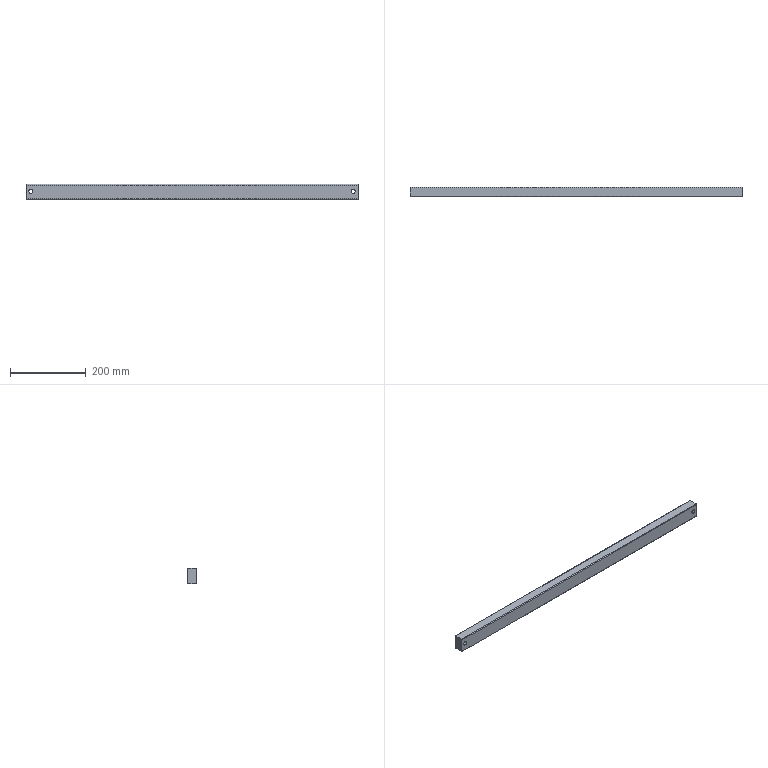Part | SolidWorks | features Cut 1, Fillet 1, Sweep 1, WeldmentFeature 1 | 1 solid | 14 faces | box 875 x 25 x 40 mm | volume 868078 mm3 | cylinder 8 | plane 6 | commonest cylinder face diameters 3.4 x4 11 x4
STEP:
#1=CARTESIAN_POINT('',(830.306,12.5,7.5));
#2=VERTEX_POINT('',#1);
#3=CARTESIAN_POINT('',(830.306,12.5,-3.5));
#4=VERTEX_POINT('',#3);
#5=CARTESIAN_POINT('',(830.306,12.5,2.));
#6=DIRECTION('',(0.,-1.,0.));
#7=DIRECTION('',(0.,0.,1.));
#8=AXIS2_PLACEMENT_3D('',#5,#6,#7);
#9=CIRCLE('',#8,5.5);
#10=EDGE_CURVE('',#2,#4,#9,.T.);
#11=ORIENTED_EDGE('',*,*,#10,.F.);
#12=CARTESIAN_POINT('',(830.306,-12.5,7.5));
#13=VERTEX_POINT('',#12);
#14=CARTESIAN_POINT('',(830.306,12.5,7.5));
#15=DIRECTION('',(0.,-1.,0.));
#16=VECTOR('',#15,1000.);
#17=LINE('',#14,#16);
#18=EDGE_CURVE('',#2,#13,#17,.T.);
#19=ORIENTED_EDGE('',*,*,#18,.T.);
#20=CARTESIAN_POINT('',(830.306,-12.5,-3.5));
#21=VERTEX_POINT('',#20);
#22=CARTESIAN_POINT('',(830.306,-12.5,2.));
#23=DIRECTION('',(0.,-1.,0.));
#24=DIRECTION('',(0.,0.,1.));
#25=AXIS2_PLACEMENT_3D('',#22,#23,#24);
#26=CIRCLE('',#25,5.5);
#27=EDGE_CURVE('',#13,#21,#26,.T.);
#28=ORIENTED_EDGE('',*,*,#27,.T.);
#29=CARTESIAN_POINT('',(830.306,12.5,-3.5));
#30=DIRECTION('',(0.,-1.,0.));
#31=VECTOR('',#30,1000.);
#32=LINE('',#29,#31);
#33=EDGE_CURVE('',#4,#21,#32,.T.);
#34=ORIENTED_EDGE('',*,*,#33,.F.);
#35=EDGE_LOOP('',(#11,#19,#28,#34));
#36=FACE_OUTER_BOUND('',#35,.T.);
#37=CARTESIAN_POINT('',(830.306,12.5,2.));
#38=DIRECTION('',(0.,-1.,0.));
#39=DIRECTION('',(0.,0.,-1.));
#40=AXIS2_PLACEMENT_3D('',#37,#38,#39);
#41=CYLINDRICAL_SURFACE('',#40,5.5);
#42=ADVANCED_FACE('',(#36),#41,.F.);
#43=CARTESIAN_POINT('',(-19.694,12.5,7.5));
#44=VERTEX_POINT('',#43);
#45=CARTESIAN_POINT('',(-19.694,12.5,-3.5));
#46=VERTEX_POINT('',#45);
#47=CARTESIAN_POINT('',(-19.694,12.5,2.));
#48=DIRECTION('',(0.,-1.,0.));
#49=DIRECTION('',(0.,0.,-1.));
#50=AXIS2_PLACEMENT_3D('',#47,#48,#49);
#51=CIRCLE('',#50,5.5);
#52=EDGE_CURVE('',#44,#46,#51,.T.);
#53=ORIENTED_EDGE('',*,*,#52,.F.);
#54=CARTESIAN_POINT('',(-19.694,-12.5,7.5));
#55=VERTEX_POINT('',#54);
#56=CARTESIAN_POINT('',(-19.694,12.5,7.5));
#57=DIRECTION('',(0.,-1.,0.));
#58=VECTOR('',#57,1000.);
#59=LINE('',#56,#58);
#60=EDGE_CURVE('',#44,#55,#59,.T.);
#61=ORIENTED_EDGE('',*,*,#60,.T.);
#62=CARTESIAN_POINT('',(-19.694,-12.5,-3.5));
#63=VERTEX_POINT('',#62);
#64=CARTESIAN_POINT('',(-19.694,-12.5,2.));
#65=DIRECTION('',(0.,-1.,0.));
#66=DIRECTION('',(0.,0.,-1.));
#67=AXIS2_PLACEMENT_3D('',#64,#65,#66);
#68=CIRCLE('',#67,5.5);
#69=EDGE_CURVE('',#55,#63,#68,.T.);
#70=ORIENTED_EDGE('',*,*,#69,.T.);
#71=CARTESIAN_POINT('',(-19.694,12.5,-3.5));
#72=DIRECTION('',(0.,-1.,0.));
#73=VECTOR('',#72,1000.);
#74=LINE('',#71,#73);
#75=EDGE_CURVE('',#46,#63,#74,.T.);
#76=ORIENTED_EDGE('',*,*,#75,.F.);
#77=EDGE_LOOP('',(#53,#61,#70,#76));
#78=FACE_OUTER_BOUND('',#77,.T.);
#79=CARTESIAN_POINT('',(-19.694,12.5,2.));
#80=DIRECTION('',(0.,-1.,0.));
#81=DIRECTION('',(0.,0.,-1.));
#82=AXIS2_PLACEMENT_3D('',#79,#80,#81);
#83=CYLINDRICAL_SURFACE('',#82,5.5);
#84=ADVANCED_FACE('',(#78),#83,.F.);
#85=CARTESIAN_POINT('',(-32.194,10.8,20.));
#86=VERTEX_POINT('',#85);
#87=CARTESIAN_POINT('',(-32.194,-10.8,20.));
#88=VERTEX_POINT('',#87);
#89=CARTESIAN_POINT('',(-32.194,12.5,20.));
#90=DIRECTION('',(0.,-1.,0.));
#91=VECTOR('',#90,1000.);
#92=LINE('',#89,#91);
#93=EDGE_CURVE('',#86,#88,#92,.T.);
#94=ORIENTED_EDGE('',*,*,#93,.T.);
#95=CARTESIAN_POINT('',(842.806,-10.8,20.));
#96=VERTEX_POINT('',#95);
#97=CARTESIAN_POINT('',(842.806,-10.8,20.));
#98=DIRECTION('',(1.,0.,0.));
#99=VECTOR('',#98,1000.);
#100=LINE('',#97,#99);
#101=EDGE_CURVE('',#88,#96,#100,.T.);
#102=ORIENTED_EDGE('',*,*,#101,.T.);
#103=CARTESIAN_POINT('',(842.806,10.8,20.));
#104=VERTEX_POINT('',#103);
#105=CARTESIAN_POINT('',(842.806,12.5,20.));
#106=DIRECTION('',(0.,-1.,0.));
#107=VECTOR('',#106,1000.);
#108=LINE('',#105,#107);
#109=EDGE_CURVE('',#104,#96,#108,.T.);
#110=ORIENTED_EDGE('',*,*,#109,.F.);
#111=CARTESIAN_POINT('',(842.806,10.8,20.));
#112=DIRECTION('',(-1.,0.,0.));
#113=VECTOR('',#112,1000.);
#114=LINE('',#111,#113);
#115=EDGE_CURVE('',#104,#86,#114,.T.);
#116=ORIENTED_EDGE('',*,*,#115,.T.);
#117=EDGE_LOOP('',(#94,#102,#110,#116));
#118=FACE_OUTER_BOUND('',#117,.T.);
#119=CARTESIAN_POINT('',(842.806,12.5,20.));
#120=DIRECTION('',(0.,0.,-1.));
#121=DIRECTION('',(0.,1.,0.));
#122=AXIS2_PLACEMENT_3D('',#119,#120,#121);
#123=PLANE('',#122);
#124=ADVANCED_FACE('',(#118),#123,.F.);
#125=CARTESIAN_POINT('',(830.306,-12.5,2.));
#126=DIRECTION('',(0.,-1.,0.));
#127=DIRECTION('',(0.,0.,1.));
#128=AXIS2_PLACEMENT_3D('',#125,#126,#127);
#129=CIRCLE('',#128,5.5);
#130=EDGE_CURVE('',#21,#13,#129,.T.);
#131=ORIENTED_EDGE('',*,*,#130,.F.);
#132=ORIENTED_EDGE('',*,*,#27,.F.);
#133=EDGE_LOOP('',(#131,#132));
#134=FACE_BOUND('',#133,.T.);
#135=CARTESIAN_POINT('',(-19.694,-12.5,2.));
#136=DIRECTION('',(0.,-1.,0.));
#137=DIRECTION('',(0.,0.,-1.));
#138=AXIS2_PLACEMENT_3D('',#135,#136,#137);
#139=CIRCLE('',#138,5.5);
#140=EDGE_CURVE('',#63,#55,#139,.T.);
#141=ORIENTED_EDGE('',*,*,#140,.F.);
#142=ORIENTED_EDGE('',*,*,#69,.F.);
#143=EDGE_LOOP('',(#141,#142));
#144=FACE_BOUND('',#143,.T.);
#145=CARTESIAN_POINT('',(-32.194,-12.5,18.3));
#146=VERTEX_POINT('',#145);
#147=CARTESIAN_POINT('',(-32.194,-12.5,-18.3));
#148=VERTEX_POINT('',#147);
#149=CARTESIAN_POINT('',(-32.194,-12.5,-20.));
#150=DIRECTION('',(0.,0.,-1.));
#151=VECTOR('',#150,1000.);
#152=LINE('',#149,#151);
#153=EDGE_CURVE('',#146,#148,#152,.T.);
#154=ORIENTED_EDGE('',*,*,#153,.T.);
#155=CARTESIAN_POINT('',(842.806,-12.5,-18.3));
#156=VERTEX_POINT('',#155);
#157=CARTESIAN_POINT('',(842.806,-12.5,-18.3));
#158=DIRECTION('',(1.,0.,0.));
#159=VECTOR('',#158,1000.);
#160=LINE('',#157,#159);
#161=EDGE_CURVE('',#148,#156,#160,.T.);
#162=ORIENTED_EDGE('',*,*,#161,.T.);
#163=CARTESIAN_POINT('',(842.806,-12.5,18.3));
#164=VERTEX_POINT('',#163);
#165=CARTESIAN_POINT('',(842.806,-12.5,-20.));
#166=DIRECTION('',(0.,0.,-1.));
#167=VECTOR('',#166,1000.);
#168=LINE('',#165,#167);
#169=EDGE_CURVE('',#164,#156,#168,.T.);
#170=ORIENTED_EDGE('',*,*,#169,.F.);
#171=CARTESIAN_POINT('',(842.806,-12.5,18.3));
#172=DIRECTION('',(-1.,0.,0.));
#173=VECTOR('',#172,1000.);
#174=LINE('',#171,#173);
#175=EDGE_CURVE('',#164,#146,#174,.T.);
#176=ORIENTED_EDGE('',*,*,#175,.T.);
#177=EDGE_LOOP('',(#154,#162,#170,#176));
#178=FACE_OUTER_BOUND('',#177,.T.);
#179=CARTESIAN_POINT('',(842.806,-12.5,-20.));
#180=DIRECTION('',(0.,1.,0.));
#181=DIRECTION('',(0.,0.,1.));
#182=AXIS2_PLACEMENT_3D('',#179,#180,#181);
#183=PLANE('',#182);
#184=ADVANCED_FACE('',(#134,#144,#178),#183,.F.);
#185=CARTESIAN_POINT('',(842.806,-10.8,-20.));
#186=VERTEX_POINT('',#185);
#187=CARTESIAN_POINT('',(842.806,10.8,-20.));
#188=VERTEX_POINT('',#187);
#189=CARTESIAN_POINT('',(842.806,12.5,-20.));
#190=DIRECTION('',(0.,1.,0.));
#191=VECTOR('',#190,1000.);
#192=LINE('',#189,#191);
#193=EDGE_CURVE('',#186,#188,#192,.T.);
#194=ORIENTED_EDGE('',*,*,#193,.F.);
#195=CARTESIAN_POINT('',(-32.194,-10.8,-20.));
#196=VERTEX_POINT('',#195);
#197=CARTESIAN_POINT('',(842.806,-10.8,-20.));
#198=DIRECTION('',(-1.,0.,0.));
#199=VECTOR('',#198,1000.);
#200=LINE('',#197,#199);
#201=EDGE_CURVE('',#186,#196,#200,.T.);
#202=ORIENTED_EDGE('',*,*,#201,.T.);
#203=CARTESIAN_POINT('',(-32.194,10.8,-20.));
#204=VERTEX_POINT('',#203);
#205=CARTESIAN_POINT('',(-32.194,12.5,-20.));
#206=DIRECTION('',(0.,1.,0.));
#207=VECTOR('',#206,1000.);
#208=LINE('',#205,#207);
#209=EDGE_CURVE('',#196,#204,#208,.T.);
#210=ORIENTED_EDGE('',*,*,#209,.T.);
#211=CARTESIAN_POINT('',(842.806,10.8,-20.));
#212=DIRECTION('',(1.,0.,0.));
#213=VECTOR('',#212,1000.);
#214=LINE('',#211,#213);
#215=EDGE_CURVE('',#204,#188,#214,.T.);
#216=ORIENTED_EDGE('',*,*,#215,.T.);
#217=EDGE_LOOP('',(#194,#202,#210,#216));
#218=FACE_OUTER_BOUND('',#217,.T.);
#219=CARTESIAN_POINT('',(842.806,12.5,-20.));
#220=DIRECTION('',(0.,0.,1.));
#221=DIRECTION('',(0.,-1.,0.));
#222=AXIS2_PLACEMENT_3D('',#219,#220,#221);
#223=PLANE('',#222);
#224=ADVANCED_FACE('',(#218),#223,.F.);
#225=CARTESIAN_POINT('',(830.306,12.5,2.));
#226=DIRECTION('',(0.,-1.,0.));
#227=DIRECTION('',(0.,0.,1.));
#228=AXIS2_PLACEMENT_3D('',#225,#226,#227);
#229=CIRCLE('',#228,5.5);
#230=EDGE_CURVE('',#4,#2,#229,.T.);
#231=ORIENTED_EDGE('',*,*,#230,.T.);
#232=ORIENTED_EDGE('',*,*,#10,.T.);
#233=EDGE_LOOP('',(#231,#232));
#234=FACE_BOUND('',#233,.T.);
#235=CARTESIAN_POINT('',(-19.694,12.5,2.));
#236=DIRECTION('',(0.,-1.,0.));
#237=DIRECTION('',(0.,0.,-1.));
#238=AXIS2_PLACEMENT_3D('',#235,#236,#237);
#239=CIRCLE('',#238,5.5);
#240=EDGE_CURVE('',#46,#44,#239,.T.);
#241=ORIENTED_EDGE('',*,*,#240,.T.);
#242=ORIENTED_EDGE('',*,*,#52,.T.);
#243=EDGE_LOOP('',(#241,#242));
#244=FACE_BOUND('',#243,.T.);
#245=CARTESIAN_POINT('',(-32.194,12.5,-18.3));
#246=VERTEX_POINT('',#245);
#247=CARTESIAN_POINT('',(-32.194,12.5,18.3));
#248=VERTEX_POINT('',#247);
#249=CARTESIAN_POINT('',(-32.194,12.5,-20.));
#250=DIRECTION('',(0.,0.,1.));
#251=VECTOR('',#250,1000.);
#252=LINE('',#249,#251);
#253=EDGE_CURVE('',#246,#248,#252,.T.);
#254=ORIENTED_EDGE('',*,*,#253,.T.);
#255=CARTESIAN_POINT('',(842.806,12.5,18.3));
#256=VERTEX_POINT('',#255);
#257=CARTESIAN_POINT('',(842.806,12.5,18.3));
#258=DIRECTION('',(1.,0.,0.));
#259=VECTOR('',#258,1000.);
#260=LINE('',#257,#259);
#261=EDGE_CURVE('',#248,#256,#260,.T.);
#262=ORIENTED_EDGE('',*,*,#261,.T.);
#263=CARTESIAN_POINT('',(842.806,12.5,-18.3));
#264=VERTEX_POINT('',#263);
#265=CARTESIAN_POINT('',(842.806,12.5,-20.));
#266=DIRECTION('',(0.,0.,1.));
#267=VECTOR('',#266,1000.);
#268=LINE('',#265,#267);
#269=EDGE_CURVE('',#264,#256,#268,.T.);
#270=ORIENTED_EDGE('',*,*,#269,.F.);
#271=CARTESIAN_POINT('',(842.806,12.5,-18.3));
#272=DIRECTION('',(-1.,0.,0.));
#273=VECTOR('',#272,1000.);
#274=LINE('',#271,#273);
#275=EDGE_CURVE('',#264,#246,#274,.T.);
#276=ORIENTED_EDGE('',*,*,#275,.T.);
#277=EDGE_LOOP('',(#254,#262,#270,#276));
#278=FACE_OUTER_BOUND('',#277,.T.);
#279=CARTESIAN_POINT('',(842.806,12.5,-20.));
#280=DIRECTION('',(0.,-1.,0.));
#281=DIRECTION('',(0.,0.,-1.));
#282=AXIS2_PLACEMENT_3D('',#279,#280,#281);
#283=PLANE('',#282);
#284=ADVANCED_FACE('',(#234,#244,#278),#283,.F.);
#285=ORIENTED_EDGE('',*,*,#169,.T.);
#286=CARTESIAN_POINT('',(842.806,-10.8,-18.3));
#287=DIRECTION('',(1.,0.,0.));
#288=DIRECTION('',(0.,0.,1.));
#289=AXIS2_PLACEMENT_3D('',#286,#287,#288);
#290=CIRCLE('',#289,1.7);
#291=EDGE_CURVE('',#156,#186,#290,.T.);
#292=ORIENTED_EDGE('',*,*,#291,.T.);
#293=ORIENTED_EDGE('',*,*,#193,.T.);
#294=CARTESIAN_POINT('',(842.806,10.8,-18.3));
#295=DIRECTION('',(1.,0.,0.));
#296=DIRECTION('',(0.,0.,1.));
#297=AXIS2_PLACEMENT_3D('',#294,#295,#296);
#298=CIRCLE('',#297,1.7);
#299=EDGE_CURVE('',#188,#264,#298,.T.);
#300=ORIENTED_EDGE('',*,*,#299,.T.);
#301=ORIENTED_EDGE('',*,*,#269,.T.);
#302=CARTESIAN_POINT('',(842.806,10.8,18.3));
#303=DIRECTION('',(1.,0.,0.));
#304=DIRECTION('',(0.,0.,1.));
#305=AXIS2_PLACEMENT_3D('',#302,#303,#304);
#306=CIRCLE('',#305,1.7);
#307=EDGE_CURVE('',#256,#104,#306,.T.);
#308=ORIENTED_EDGE('',*,*,#307,.T.);
#309=ORIENTED_EDGE('',*,*,#109,.T.);
#310=CARTESIAN_POINT('',(842.806,-10.8,18.3));
#311=DIRECTION('',(1.,0.,0.));
#312=DIRECTION('',(0.,0.,1.));
#313=AXIS2_PLACEMENT_3D('',#310,#311,#312);
#314=CIRCLE('',#313,1.7);
#315=EDGE_CURVE('',#96,#164,#314,.T.);
#316=ORIENTED_EDGE('',*,*,#315,.T.);
#317=EDGE_LOOP('',(#285,#292,#293,#300,#301,#308,#309,#316));
#318=FACE_OUTER_BOUND('',#317,.T.);
#319=CARTESIAN_POINT('',(842.806,0.,0.));
#320=DIRECTION('',(-1.,0.,0.));
#321=DIRECTION('',(0.,0.,1.));
#322=AXIS2_PLACEMENT_3D('',#319,#320,#321);
#323=PLANE('',#322);
#324=ADVANCED_FACE('',(#318),#323,.F.);
#325=ORIENTED_EDGE('',*,*,#209,.F.);
#326=CARTESIAN_POINT('',(-32.194,-10.8,-18.3));
#327=DIRECTION('',(-1.,0.,0.));
#328=DIRECTION('',(0.,0.,1.));
#329=AXIS2_PLACEMENT_3D('',#326,#327,#328);
#330=CIRCLE('',#329,1.7);
#331=EDGE_CURVE('',#196,#148,#330,.T.);
#332=ORIENTED_EDGE('',*,*,#331,.T.);
#333=ORIENTED_EDGE('',*,*,#153,.F.);
#334=CARTESIAN_POINT('',(-32.194,-10.8,18.3));
#335=DIRECTION('',(-1.,0.,0.));
#336=DIRECTION('',(0.,0.,1.));
#337=AXIS2_PLACEMENT_3D('',#334,#335,#336);
#338=CIRCLE('',#337,1.7);
#339=EDGE_CURVE('',#146,#88,#338,.T.);
#340=ORIENTED_EDGE('',*,*,#339,.T.);
#341=ORIENTED_EDGE('',*,*,#93,.F.);
#342=CARTESIAN_POINT('',(-32.194,10.8,18.3));
#343=DIRECTION('',(-1.,0.,0.));
#344=DIRECTION('',(0.,0.,1.));
#345=AXIS2_PLACEMENT_3D('',#342,#343,#344);
#346=CIRCLE('',#345,1.7);
#347=EDGE_CURVE('',#86,#248,#346,.T.);
#348=ORIENTED_EDGE('',*,*,#347,.T.);
#349=ORIENTED_EDGE('',*,*,#253,.F.);
#350=CARTESIAN_POINT('',(-32.194,10.8,-18.3));
#351=DIRECTION('',(-1.,0.,0.));
#352=DIRECTION('',(0.,0.,1.));
#353=AXIS2_PLACEMENT_3D('',#350,#351,#352);
#354=CIRCLE('',#353,1.7);
#355=EDGE_CURVE('',#246,#204,#354,.T.);
#356=ORIENTED_EDGE('',*,*,#355,.T.);
#357=EDGE_LOOP('',(#325,#332,#333,#340,#341,#348,#349,#356));
#358=FACE_OUTER_BOUND('',#357,.T.);
#359=CARTESIAN_POINT('',(-32.194,0.,0.));
#360=DIRECTION('',(-1.,0.,0.));
#361=DIRECTION('',(0.,0.,1.));
#362=AXIS2_PLACEMENT_3D('',#359,#360,#361);
#363=PLANE('',#362);
#364=ADVANCED_FACE('',(#358),#363,.T.);
#365=ORIENTED_EDGE('',*,*,#291,.F.);
#366=ORIENTED_EDGE('',*,*,#161,.F.);
#367=ORIENTED_EDGE('',*,*,#331,.F.);
#368=ORIENTED_EDGE('',*,*,#201,.F.);
#369=EDGE_LOOP('',(#365,#366,#367,#368));
#370=FACE_OUTER_BOUND('',#369,.T.);
#371=CARTESIAN_POINT('',(842.806,-10.8,-18.3));
#372=DIRECTION('',(-1.,0.,0.));
#373=DIRECTION('',(0.,0.,1.));
#374=AXIS2_PLACEMENT_3D('',#371,#372,#373);
#375=CYLINDRICAL_SURFACE('',#374,1.7);
#376=ADVANCED_FACE('',(#370),#375,.T.);
#377=ORIENTED_EDGE('',*,*,#315,.F.);
#378=ORIENTED_EDGE('',*,*,#101,.F.);
#379=ORIENTED_EDGE('',*,*,#339,.F.);
#380=ORIENTED_EDGE('',*,*,#175,.F.);
#381=EDGE_LOOP('',(#377,#378,#379,#380));
#382=FACE_OUTER_BOUND('',#381,.T.);
#383=CARTESIAN_POINT('',(842.806,-10.8,18.3));
#384=DIRECTION('',(-1.,0.,0.));
#385=DIRECTION('',(0.,0.,1.));
#386=AXIS2_PLACEMENT_3D('',#383,#384,#385);
#387=CYLINDRICAL_SURFACE('',#386,1.7);
#388=ADVANCED_FACE('',(#382),#387,.T.);
#389=ORIENTED_EDGE('',*,*,#307,.F.);
#390=ORIENTED_EDGE('',*,*,#261,.F.);
#391=ORIENTED_EDGE('',*,*,#347,.F.);
#392=ORIENTED_EDGE('',*,*,#115,.F.);
#393=EDGE_LOOP('',(#389,#390,#391,#392));
#394=FACE_OUTER_BOUND('',#393,.T.);
#395=CARTESIAN_POINT('',(842.806,10.8,18.3));
#396=DIRECTION('',(-1.,0.,0.));
#397=DIRECTION('',(0.,0.,1.));
#398=AXIS2_PLACEMENT_3D('',#395,#396,#397);
#399=CYLINDRICAL_SURFACE('',#398,1.7);
#400=ADVANCED_FACE('',(#394),#399,.T.);
#401=ORIENTED_EDGE('',*,*,#299,.F.);
#402=ORIENTED_EDGE('',*,*,#215,.F.);
#403=ORIENTED_EDGE('',*,*,#355,.F.);
#404=ORIENTED_EDGE('',*,*,#275,.F.);
#405=EDGE_LOOP('',(#401,#402,#403,#404));
#406=FACE_OUTER_BOUND('',#405,.T.);
#407=CARTESIAN_POINT('',(842.806,10.8,-18.3));
#408=DIRECTION('',(-1.,0.,0.));
#409=DIRECTION('',(0.,0.,1.));
#410=AXIS2_PLACEMENT_3D('',#407,#408,#409);
#411=CYLINDRICAL_SURFACE('',#410,1.7);
#412=ADVANCED_FACE('',(#406),#411,.T.);
#413=ORIENTED_EDGE('',*,*,#60,.F.);
#414=ORIENTED_EDGE('',*,*,#240,.F.);
#415=ORIENTED_EDGE('',*,*,#75,.T.);
#416=ORIENTED_EDGE('',*,*,#140,.T.);
#417=EDGE_LOOP('',(#413,#414,#415,#416));
#418=FACE_OUTER_BOUND('',#417,.T.);
#419=CARTESIAN_POINT('',(-19.694,12.5,2.));
#420=DIRECTION('',(0.,-1.,0.));
#421=DIRECTION('',(0.,0.,-1.));
#422=AXIS2_PLACEMENT_3D('',#419,#420,#421);
#423=CYLINDRICAL_SURFACE('',#422,5.5);
#424=ADVANCED_FACE('',(#418),#423,.F.);
#425=ORIENTED_EDGE('',*,*,#18,.F.);
#426=ORIENTED_EDGE('',*,*,#230,.F.);
#427=ORIENTED_EDGE('',*,*,#33,.T.);
#428=ORIENTED_EDGE('',*,*,#130,.T.);
#429=EDGE_LOOP('',(#425,#426,#427,#428));
#430=FACE_OUTER_BOUND('',#429,.T.);
#431=CARTESIAN_POINT('',(830.306,12.5,2.));
#432=DIRECTION('',(0.,-1.,0.));
#433=DIRECTION('',(0.,0.,-1.));
#434=AXIS2_PLACEMENT_3D('',#431,#432,#433);
#435=CYLINDRICAL_SURFACE('',#434,5.5);
#436=ADVANCED_FACE('',(#430),#435,.F.);
#437=CLOSED_SHELL('',(#42,#84,#124,#184,#224,#284,#324,#364,#376,#388,#400,#412,#424,#436));
#438=MANIFOLD_SOLID_BREP('',#437);
#439=CARTESIAN_POINT('',(0.,0.,0.));
#440=DIRECTION('',(0.,0.,1.));
#441=DIRECTION('',(1.,0.,0.));
#442=AXIS2_PLACEMENT_3D('',#439,#440,#441);
#443=(LENGTH_UNIT()NAMED_UNIT(*)SI_UNIT(.MILLI.,.METRE.));
#444=UNCERTAINTY_MEASURE_WITH_UNIT(LENGTH_MEASURE(0.00001),#443,'','');
#445=(NAMED_UNIT(*)PLANE_ANGLE_UNIT()SI_UNIT($,.RADIAN.));
#446=(NAMED_UNIT(*)SI_UNIT($,.STERADIAN.)SOLID_ANGLE_UNIT());
#447=(GEOMETRIC_REPRESENTATION_CONTEXT(3)GLOBAL_UNCERTAINTY_ASSIGNED_CONTEXT((#444))GLOBAL_UNIT_ASSIGNED_CONTEXT((#443,#445,#446))REPRESENTATION_CONTEXT('',''));
#448=ADVANCED_BREP_SHAPE_REPRESENTATION('',(#438,#442),#447);